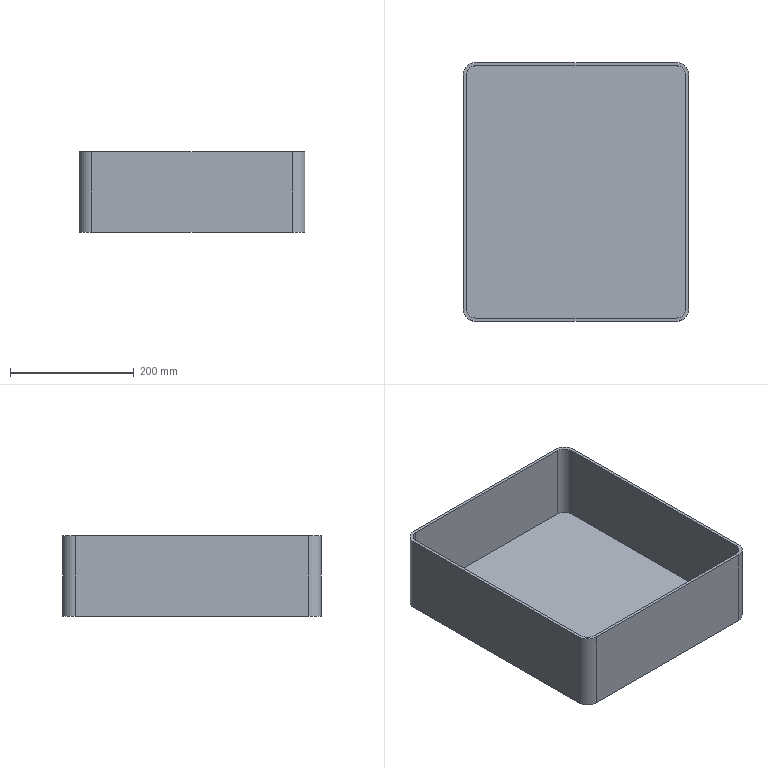Part | NX | features solid 2 | 1 solid | 19 faces | box 364.214 x 417 x 130 mm | volume 1702910 mm3 | plane 11 | cylinder 8 | commonest cylinder face diameters 30 x4 40 x4
STEP:
#1=CARTESIAN_POINT('',(-163.582,-691.316,-27.));
#2=VERTEX_POINT('',#1);
#3=CARTESIAN_POINT('',(160.632,-691.316,-27.));
#4=VERTEX_POINT('',#3);
#5=CARTESIAN_POINT('',(-1.475,-691.316,-27.));
#6=DIRECTION('',(-1.,0.,0.));
#7=VECTOR('',#6,1000.);
#8=LINE('',#5,#7);
#9=EDGE_CURVE('',#2,#4,#8,.F.);
#10=ORIENTED_EDGE('',*,*,#9,.F.);
#11=CARTESIAN_POINT('',(-183.582,-711.316,-27.));
#12=VERTEX_POINT('',#11);
#13=CARTESIAN_POINT('',(-163.582,-711.316,-27.));
#14=DIRECTION('',(0.,0.,-1.));
#15=DIRECTION('',(-1.,0.,0.));
#16=AXIS2_PLACEMENT_3D('',#13,#14,#15);
#17=CIRCLE('',#16,20.);
#18=EDGE_CURVE('',#2,#12,#17,.F.);
#19=ORIENTED_EDGE('',*,*,#18,.T.);
#20=CARTESIAN_POINT('',(-183.582,-1088.316,-27.));
#21=VERTEX_POINT('',#20);
#22=CARTESIAN_POINT('',(-183.582,-899.816,-27.));
#23=DIRECTION('',(0.,-1.,0.));
#24=VECTOR('',#23,1000.);
#25=LINE('',#22,#24);
#26=EDGE_CURVE('',#21,#12,#25,.F.);
#27=ORIENTED_EDGE('',*,*,#26,.F.);
#28=CARTESIAN_POINT('',(-163.582,-1108.316,-27.));
#29=VERTEX_POINT('',#28);
#30=CARTESIAN_POINT('',(-163.582,-1088.316,-27.));
#31=DIRECTION('',(0.,0.,-1.));
#32=DIRECTION('',(-1.,0.,0.));
#33=AXIS2_PLACEMENT_3D('',#30,#31,#32);
#34=CIRCLE('',#33,20.);
#35=EDGE_CURVE('',#21,#29,#34,.F.);
#36=ORIENTED_EDGE('',*,*,#35,.T.);
#37=CARTESIAN_POINT('',(160.632,-1108.316,-27.));
#38=VERTEX_POINT('',#37);
#39=CARTESIAN_POINT('',(-1.475,-1108.316,-27.));
#40=DIRECTION('',(1.,0.,0.));
#41=VECTOR('',#40,1000.);
#42=LINE('',#39,#41);
#43=EDGE_CURVE('',#38,#29,#42,.F.);
#44=ORIENTED_EDGE('',*,*,#43,.F.);
#45=CARTESIAN_POINT('',(180.632,-1088.316,-27.));
#46=VERTEX_POINT('',#45);
#47=CARTESIAN_POINT('',(160.632,-1088.316,-27.));
#48=DIRECTION('',(0.,0.,-1.));
#49=DIRECTION('',(-1.,0.,0.));
#50=AXIS2_PLACEMENT_3D('',#47,#48,#49);
#51=CIRCLE('',#50,20.);
#52=EDGE_CURVE('',#38,#46,#51,.F.);
#53=ORIENTED_EDGE('',*,*,#52,.T.);
#54=CARTESIAN_POINT('',(180.632,-711.316,-27.));
#55=VERTEX_POINT('',#54);
#56=CARTESIAN_POINT('',(180.632,-899.816,-27.));
#57=DIRECTION('',(0.,1.,0.));
#58=VECTOR('',#57,1000.);
#59=LINE('',#56,#58);
#60=EDGE_CURVE('',#55,#46,#59,.F.);
#61=ORIENTED_EDGE('',*,*,#60,.F.);
#62=CARTESIAN_POINT('',(160.632,-711.316,-27.));
#63=DIRECTION('',(0.,0.,-1.));
#64=DIRECTION('',(-1.,0.,0.));
#65=AXIS2_PLACEMENT_3D('',#62,#63,#64);
#66=CIRCLE('',#65,20.);
#67=EDGE_CURVE('',#55,#4,#66,.F.);
#68=ORIENTED_EDGE('',*,*,#67,.T.);
#69=EDGE_LOOP('',(#10,#19,#27,#36,#44,#53,#61,#68));
#70=FACE_BOUND('',#69,.T.);
#71=CARTESIAN_POINT('',(-163.582,-696.316,-27.));
#72=VERTEX_POINT('',#71);
#73=CARTESIAN_POINT('',(-178.582,-711.316,-27.));
#74=VERTEX_POINT('',#73);
#75=CARTESIAN_POINT('',(-163.582,-711.316,-27.));
#76=DIRECTION('',(0.,0.,-1.));
#77=DIRECTION('',(-1.,0.,0.));
#78=AXIS2_PLACEMENT_3D('',#75,#76,#77);
#79=CIRCLE('',#78,15.);
#80=EDGE_CURVE('',#72,#74,#79,.F.);
#81=ORIENTED_EDGE('',*,*,#80,.F.);
#82=CARTESIAN_POINT('',(160.632,-696.316,-27.));
#83=VERTEX_POINT('',#82);
#84=CARTESIAN_POINT('',(-1.475,-696.316,-27.));
#85=DIRECTION('',(-1.,0.,0.));
#86=VECTOR('',#85,1000.);
#87=LINE('',#84,#86);
#88=EDGE_CURVE('',#72,#83,#87,.F.);
#89=ORIENTED_EDGE('',*,*,#88,.T.);
#90=CARTESIAN_POINT('',(175.632,-711.316,-27.));
#91=VERTEX_POINT('',#90);
#92=CARTESIAN_POINT('',(160.632,-711.316,-27.));
#93=DIRECTION('',(0.,0.,-1.));
#94=DIRECTION('',(-1.,0.,0.));
#95=AXIS2_PLACEMENT_3D('',#92,#93,#94);
#96=CIRCLE('',#95,15.);
#97=EDGE_CURVE('',#91,#83,#96,.F.);
#98=ORIENTED_EDGE('',*,*,#97,.F.);
#99=CARTESIAN_POINT('',(175.632,-1088.316,-27.));
#100=VERTEX_POINT('',#99);
#101=CARTESIAN_POINT('',(175.632,-899.816,-27.));
#102=DIRECTION('',(0.,1.,0.));
#103=VECTOR('',#102,1000.);
#104=LINE('',#101,#103);
#105=EDGE_CURVE('',#91,#100,#104,.F.);
#106=ORIENTED_EDGE('',*,*,#105,.T.);
#107=CARTESIAN_POINT('',(160.632,-1103.316,-27.));
#108=VERTEX_POINT('',#107);
#109=CARTESIAN_POINT('',(160.632,-1088.316,-27.));
#110=DIRECTION('',(0.,0.,-1.));
#111=DIRECTION('',(-1.,0.,0.));
#112=AXIS2_PLACEMENT_3D('',#109,#110,#111);
#113=CIRCLE('',#112,15.);
#114=EDGE_CURVE('',#108,#100,#113,.F.);
#115=ORIENTED_EDGE('',*,*,#114,.F.);
#116=CARTESIAN_POINT('',(-163.582,-1103.316,-27.));
#117=VERTEX_POINT('',#116);
#118=CARTESIAN_POINT('',(-1.475,-1103.316,-27.));
#119=DIRECTION('',(1.,0.,0.));
#120=VECTOR('',#119,1000.);
#121=LINE('',#118,#120);
#122=EDGE_CURVE('',#108,#117,#121,.F.);
#123=ORIENTED_EDGE('',*,*,#122,.T.);
#124=CARTESIAN_POINT('',(-178.582,-1088.316,-27.));
#125=VERTEX_POINT('',#124);
#126=CARTESIAN_POINT('',(-163.582,-1088.316,-27.));
#127=DIRECTION('',(0.,0.,-1.));
#128=DIRECTION('',(-1.,0.,0.));
#129=AXIS2_PLACEMENT_3D('',#126,#127,#128);
#130=CIRCLE('',#129,15.);
#131=EDGE_CURVE('',#125,#117,#130,.F.);
#132=ORIENTED_EDGE('',*,*,#131,.F.);
#133=CARTESIAN_POINT('',(-178.582,-899.816,-27.));
#134=DIRECTION('',(0.,-1.,0.));
#135=VECTOR('',#134,1000.);
#136=LINE('',#133,#135);
#137=EDGE_CURVE('',#125,#74,#136,.F.);
#138=ORIENTED_EDGE('',*,*,#137,.T.);
#139=EDGE_LOOP('',(#81,#89,#98,#106,#115,#123,#132,#138));
#140=FACE_BOUND('',#139,.T.);
#141=CARTESIAN_POINT('',(193.825,-479.612,-27.));
#142=DIRECTION('',(0.,0.,-1.));
#143=DIRECTION('',(0.,1.,0.));
#144=AXIS2_PLACEMENT_3D('',#141,#142,#143);
#145=PLANE('',#144);
#146=ADVANCED_FACE('',(#70,#140),#145,.F.);
#147=CARTESIAN_POINT('',(-163.582,-1108.316,-157.));
#148=VERTEX_POINT('',#147);
#149=CARTESIAN_POINT('',(160.632,-1108.316,-157.));
#150=VERTEX_POINT('',#149);
#151=CARTESIAN_POINT('',(-1.475,-1108.316,-157.));
#152=DIRECTION('',(-1.,0.,0.));
#153=VECTOR('',#152,1000.);
#154=LINE('',#151,#153);
#155=EDGE_CURVE('',#148,#150,#154,.F.);
#156=ORIENTED_EDGE('',*,*,#155,.T.);
#157=CARTESIAN_POINT('',(160.632,-1108.316,-187.));
#158=DIRECTION('',(0.,0.,1.));
#159=VECTOR('',#158,1000.);
#160=LINE('',#157,#159);
#161=EDGE_CURVE('',#150,#38,#160,.T.);
#162=ORIENTED_EDGE('',*,*,#161,.T.);
#163=ORIENTED_EDGE('',*,*,#43,.T.);
#164=CARTESIAN_POINT('',(-163.582,-1108.316,-187.));
#165=DIRECTION('',(0.,0.,1.));
#166=VECTOR('',#165,1000.);
#167=LINE('',#164,#166);
#168=EDGE_CURVE('',#29,#148,#167,.F.);
#169=ORIENTED_EDGE('',*,*,#168,.T.);
#170=EDGE_LOOP('',(#156,#162,#163,#169));
#171=FACE_BOUND('',#170,.T.);
#172=CARTESIAN_POINT('',(-1.475,-1108.316,-187.));
#173=DIRECTION('',(0.,-1.,0.));
#174=DIRECTION('',(0.,0.,-1.));
#175=AXIS2_PLACEMENT_3D('',#172,#173,#174);
#176=PLANE('',#175);
#177=ADVANCED_FACE('',(#171),#176,.T.);
#178=ORIENTED_EDGE('',*,*,#26,.T.);
#179=CARTESIAN_POINT('',(-183.582,-711.316,-157.));
#180=VERTEX_POINT('',#179);
#181=CARTESIAN_POINT('',(-183.582,-711.316,-187.));
#182=DIRECTION('',(0.,0.,1.));
#183=VECTOR('',#182,1000.);
#184=LINE('',#181,#183);
#185=EDGE_CURVE('',#12,#180,#184,.F.);
#186=ORIENTED_EDGE('',*,*,#185,.T.);
#187=CARTESIAN_POINT('',(-183.582,-1088.316,-157.));
#188=VERTEX_POINT('',#187);
#189=CARTESIAN_POINT('',(-183.582,-899.816,-157.));
#190=DIRECTION('',(0.,1.,0.));
#191=VECTOR('',#190,1000.);
#192=LINE('',#189,#191);
#193=EDGE_CURVE('',#180,#188,#192,.F.);
#194=ORIENTED_EDGE('',*,*,#193,.T.);
#195=CARTESIAN_POINT('',(-183.582,-1088.316,-187.));
#196=DIRECTION('',(0.,0.,1.));
#197=VECTOR('',#196,1000.);
#198=LINE('',#195,#197);
#199=EDGE_CURVE('',#188,#21,#198,.T.);
#200=ORIENTED_EDGE('',*,*,#199,.T.);
#201=EDGE_LOOP('',(#178,#186,#194,#200));
#202=FACE_BOUND('',#201,.T.);
#203=CARTESIAN_POINT('',(-183.582,-899.816,-187.));
#204=DIRECTION('',(-1.,0.,0.));
#205=DIRECTION('',(0.,0.,1.));
#206=AXIS2_PLACEMENT_3D('',#203,#204,#205);
#207=PLANE('',#206);
#208=ADVANCED_FACE('',(#202),#207,.T.);
#209=CARTESIAN_POINT('',(160.632,-691.316,-157.));
#210=VERTEX_POINT('',#209);
#211=CARTESIAN_POINT('',(-163.582,-691.316,-157.));
#212=VERTEX_POINT('',#211);
#213=CARTESIAN_POINT('',(-1.475,-691.316,-157.));
#214=DIRECTION('',(1.,0.,0.));
#215=VECTOR('',#214,1000.);
#216=LINE('',#213,#215);
#217=EDGE_CURVE('',#210,#212,#216,.F.);
#218=ORIENTED_EDGE('',*,*,#217,.T.);
#219=CARTESIAN_POINT('',(-163.582,-691.316,-187.));
#220=DIRECTION('',(0.,0.,1.));
#221=VECTOR('',#220,1000.);
#222=LINE('',#219,#221);
#223=EDGE_CURVE('',#212,#2,#222,.T.);
#224=ORIENTED_EDGE('',*,*,#223,.T.);
#225=ORIENTED_EDGE('',*,*,#9,.T.);
#226=CARTESIAN_POINT('',(160.632,-691.316,-187.));
#227=DIRECTION('',(0.,0.,1.));
#228=VECTOR('',#227,1000.);
#229=LINE('',#226,#228);
#230=EDGE_CURVE('',#4,#210,#229,.F.);
#231=ORIENTED_EDGE('',*,*,#230,.T.);
#232=EDGE_LOOP('',(#218,#224,#225,#231));
#233=FACE_BOUND('',#232,.T.);
#234=CARTESIAN_POINT('',(-1.475,-691.316,-187.));
#235=DIRECTION('',(0.,1.,0.));
#236=DIRECTION('',(0.,0.,1.));
#237=AXIS2_PLACEMENT_3D('',#234,#235,#236);
#238=PLANE('',#237);
#239=ADVANCED_FACE('',(#233),#238,.T.);
#240=ORIENTED_EDGE('',*,*,#193,.F.);
#241=CARTESIAN_POINT('',(-163.582,-711.316,-157.));
#242=DIRECTION('',(0.,0.,1.));
#243=DIRECTION('',(1.,0.,0.));
#244=AXIS2_PLACEMENT_3D('',#241,#242,#243);
#245=CIRCLE('',#244,20.);
#246=EDGE_CURVE('',#180,#212,#245,.F.);
#247=ORIENTED_EDGE('',*,*,#246,.T.);
#248=ORIENTED_EDGE('',*,*,#217,.F.);
#249=CARTESIAN_POINT('',(180.632,-711.316,-157.));
#250=VERTEX_POINT('',#249);
#251=CARTESIAN_POINT('',(160.632,-711.316,-157.));
#252=DIRECTION('',(0.,0.,1.));
#253=DIRECTION('',(1.,0.,0.));
#254=AXIS2_PLACEMENT_3D('',#251,#252,#253);
#255=CIRCLE('',#254,20.);
#256=EDGE_CURVE('',#210,#250,#255,.F.);
#257=ORIENTED_EDGE('',*,*,#256,.T.);
#258=CARTESIAN_POINT('',(180.632,-1088.316,-157.));
#259=VERTEX_POINT('',#258);
#260=CARTESIAN_POINT('',(180.632,-899.816,-157.));
#261=DIRECTION('',(0.,-1.,0.));
#262=VECTOR('',#261,1000.);
#263=LINE('',#260,#262);
#264=EDGE_CURVE('',#259,#250,#263,.F.);
#265=ORIENTED_EDGE('',*,*,#264,.F.);
#266=CARTESIAN_POINT('',(160.632,-1088.316,-157.));
#267=DIRECTION('',(0.,0.,1.));
#268=DIRECTION('',(1.,0.,0.));
#269=AXIS2_PLACEMENT_3D('',#266,#267,#268);
#270=CIRCLE('',#269,20.);
#271=EDGE_CURVE('',#259,#150,#270,.F.);
#272=ORIENTED_EDGE('',*,*,#271,.T.);
#273=ORIENTED_EDGE('',*,*,#155,.F.);
#274=CARTESIAN_POINT('',(-163.582,-1088.316,-157.));
#275=DIRECTION('',(0.,0.,1.));
#276=DIRECTION('',(1.,0.,0.));
#277=AXIS2_PLACEMENT_3D('',#274,#275,#276);
#278=CIRCLE('',#277,20.);
#279=EDGE_CURVE('',#148,#188,#278,.F.);
#280=ORIENTED_EDGE('',*,*,#279,.T.);
#281=EDGE_LOOP('',(#240,#247,#248,#257,#265,#272,#273,#280));
#282=FACE_BOUND('',#281,.T.);
#283=CARTESIAN_POINT('',(174.525,-16.,-157.));
#284=DIRECTION('',(0.,0.,1.));
#285=DIRECTION('',(-1.,0.,0.));
#286=AXIS2_PLACEMENT_3D('',#283,#284,#285);
#287=PLANE('',#286);
#288=ADVANCED_FACE('',(#282),#287,.F.);
#289=ORIENTED_EDGE('',*,*,#264,.T.);
#290=CARTESIAN_POINT('',(180.632,-711.316,-187.));
#291=DIRECTION('',(0.,0.,1.));
#292=VECTOR('',#291,1000.);
#293=LINE('',#290,#292);
#294=EDGE_CURVE('',#250,#55,#293,.T.);
#295=ORIENTED_EDGE('',*,*,#294,.T.);
#296=ORIENTED_EDGE('',*,*,#60,.T.);
#297=CARTESIAN_POINT('',(180.632,-1088.316,-187.));
#298=DIRECTION('',(0.,0.,1.));
#299=VECTOR('',#298,1000.);
#300=LINE('',#297,#299);
#301=EDGE_CURVE('',#46,#259,#300,.F.);
#302=ORIENTED_EDGE('',*,*,#301,.T.);
#303=EDGE_LOOP('',(#289,#295,#296,#302));
#304=FACE_BOUND('',#303,.T.);
#305=CARTESIAN_POINT('',(180.632,-899.816,-187.));
#306=DIRECTION('',(1.,0.,0.));
#307=DIRECTION('',(0.,0.,-1.));
#308=AXIS2_PLACEMENT_3D('',#305,#306,#307);
#309=PLANE('',#308);
#310=ADVANCED_FACE('',(#304),#309,.T.);
#311=ORIENTED_EDGE('',*,*,#246,.F.);
#312=ORIENTED_EDGE('',*,*,#185,.F.);
#313=ORIENTED_EDGE('',*,*,#18,.F.);
#314=ORIENTED_EDGE('',*,*,#223,.F.);
#315=EDGE_LOOP('',(#311,#312,#313,#314));
#316=FACE_BOUND('',#315,.T.);
#317=CARTESIAN_POINT('',(-163.582,-711.316,-187.));
#318=DIRECTION('',(0.,0.,1.));
#319=DIRECTION('',(1.,0.,0.));
#320=AXIS2_PLACEMENT_3D('',#317,#318,#319);
#321=CYLINDRICAL_SURFACE('',#320,20.);
#322=ADVANCED_FACE('',(#316),#321,.T.);
#323=ORIENTED_EDGE('',*,*,#256,.F.);
#324=ORIENTED_EDGE('',*,*,#230,.F.);
#325=ORIENTED_EDGE('',*,*,#67,.F.);
#326=ORIENTED_EDGE('',*,*,#294,.F.);
#327=EDGE_LOOP('',(#323,#324,#325,#326));
#328=FACE_BOUND('',#327,.T.);
#329=CARTESIAN_POINT('',(160.632,-711.316,-187.));
#330=DIRECTION('',(0.,0.,1.));
#331=DIRECTION('',(1.,0.,0.));
#332=AXIS2_PLACEMENT_3D('',#329,#330,#331);
#333=CYLINDRICAL_SURFACE('',#332,20.);
#334=ADVANCED_FACE('',(#328),#333,.T.);
#335=ORIENTED_EDGE('',*,*,#271,.F.);
#336=ORIENTED_EDGE('',*,*,#301,.F.);
#337=ORIENTED_EDGE('',*,*,#52,.F.);
#338=ORIENTED_EDGE('',*,*,#161,.F.);
#339=EDGE_LOOP('',(#335,#336,#337,#338));
#340=FACE_BOUND('',#339,.T.);
#341=CARTESIAN_POINT('',(160.632,-1088.316,-187.));
#342=DIRECTION('',(0.,0.,1.));
#343=DIRECTION('',(1.,0.,0.));
#344=AXIS2_PLACEMENT_3D('',#341,#342,#343);
#345=CYLINDRICAL_SURFACE('',#344,20.);
#346=ADVANCED_FACE('',(#340),#345,.T.);
#347=ORIENTED_EDGE('',*,*,#279,.F.);
#348=ORIENTED_EDGE('',*,*,#168,.F.);
#349=ORIENTED_EDGE('',*,*,#35,.F.);
#350=ORIENTED_EDGE('',*,*,#199,.F.);
#351=EDGE_LOOP('',(#347,#348,#349,#350));
#352=FACE_BOUND('',#351,.T.);
#353=CARTESIAN_POINT('',(-163.582,-1088.316,-187.));
#354=DIRECTION('',(0.,0.,1.));
#355=DIRECTION('',(1.,0.,0.));
#356=AXIS2_PLACEMENT_3D('',#353,#354,#355);
#357=CYLINDRICAL_SURFACE('',#356,20.);
#358=ADVANCED_FACE('',(#352),#357,.T.);
#359=CARTESIAN_POINT('',(-163.582,-1103.316,-152.));
#360=VERTEX_POINT('',#359);
#361=CARTESIAN_POINT('',(160.632,-1103.316,-152.));
#362=VERTEX_POINT('',#361);
#363=CARTESIAN_POINT('',(-1.475,-1103.316,-152.));
#364=DIRECTION('',(-1.,0.,0.));
#365=VECTOR('',#364,1000.);
#366=LINE('',#363,#365);
#367=EDGE_CURVE('',#360,#362,#366,.F.);
#368=ORIENTED_EDGE('',*,*,#367,.F.);
#369=CARTESIAN_POINT('',(-163.582,-1103.316,-187.));
#370=DIRECTION('',(0.,0.,-1.));
#371=VECTOR('',#370,1000.);
#372=LINE('',#369,#371);
#373=EDGE_CURVE('',#117,#360,#372,.T.);
#374=ORIENTED_EDGE('',*,*,#373,.F.);
#375=ORIENTED_EDGE('',*,*,#122,.F.);
#376=CARTESIAN_POINT('',(160.632,-1103.316,-187.));
#377=DIRECTION('',(0.,0.,-1.));
#378=VECTOR('',#377,1000.);
#379=LINE('',#376,#378);
#380=EDGE_CURVE('',#362,#108,#379,.F.);
#381=ORIENTED_EDGE('',*,*,#380,.F.);
#382=EDGE_LOOP('',(#368,#374,#375,#381));
#383=FACE_BOUND('',#382,.T.);
#384=CARTESIAN_POINT('',(-1.475,-1103.316,-187.));
#385=DIRECTION('',(0.,-1.,0.));
#386=DIRECTION('',(0.,0.,-1.));
#387=AXIS2_PLACEMENT_3D('',#384,#385,#386);
#388=PLANE('',#387);
#389=ADVANCED_FACE('',(#383),#388,.F.);
#390=ORIENTED_EDGE('',*,*,#137,.F.);
#391=CARTESIAN_POINT('',(-178.582,-1088.316,-152.));
#392=VERTEX_POINT('',#391);
#393=CARTESIAN_POINT('',(-178.582,-1088.316,-187.));
#394=DIRECTION('',(0.,0.,1.));
#395=VECTOR('',#394,1000.);
#396=LINE('',#393,#395);
#397=EDGE_CURVE('',#392,#125,#396,.T.);
#398=ORIENTED_EDGE('',*,*,#397,.F.);
#399=CARTESIAN_POINT('',(-178.582,-711.316,-152.));
#400=VERTEX_POINT('',#399);
#401=CARTESIAN_POINT('',(-178.582,-899.816,-152.));
#402=DIRECTION('',(0.,1.,0.));
#403=VECTOR('',#402,1000.);
#404=LINE('',#401,#403);
#405=EDGE_CURVE('',#400,#392,#404,.F.);
#406=ORIENTED_EDGE('',*,*,#405,.F.);
#407=CARTESIAN_POINT('',(-178.582,-711.316,-187.));
#408=DIRECTION('',(0.,0.,1.));
#409=VECTOR('',#408,1000.);
#410=LINE('',#407,#409);
#411=EDGE_CURVE('',#74,#400,#410,.F.);
#412=ORIENTED_EDGE('',*,*,#411,.F.);
#413=EDGE_LOOP('',(#390,#398,#406,#412));
#414=FACE_BOUND('',#413,.T.);
#415=CARTESIAN_POINT('',(-178.582,-899.816,-187.));
#416=DIRECTION('',(-1.,0.,0.));
#417=DIRECTION('',(0.,0.,1.));
#418=AXIS2_PLACEMENT_3D('',#415,#416,#417);
#419=PLANE('',#418);
#420=ADVANCED_FACE('',(#414),#419,.F.);
#421=CARTESIAN_POINT('',(160.632,-696.316,-152.));
#422=VERTEX_POINT('',#421);
#423=CARTESIAN_POINT('',(-163.582,-696.316,-152.));
#424=VERTEX_POINT('',#423);
#425=CARTESIAN_POINT('',(-1.475,-696.316,-152.));
#426=DIRECTION('',(1.,0.,0.));
#427=VECTOR('',#426,1000.);
#428=LINE('',#425,#427);
#429=EDGE_CURVE('',#422,#424,#428,.F.);
#430=ORIENTED_EDGE('',*,*,#429,.F.);
#431=CARTESIAN_POINT('',(160.632,-696.316,-187.));
#432=DIRECTION('',(0.,0.,1.));
#433=VECTOR('',#432,1000.);
#434=LINE('',#431,#433);
#435=EDGE_CURVE('',#83,#422,#434,.F.);
#436=ORIENTED_EDGE('',*,*,#435,.F.);
#437=ORIENTED_EDGE('',*,*,#88,.F.);
#438=CARTESIAN_POINT('',(-163.582,-696.316,-187.));
#439=DIRECTION('',(0.,0.,1.));
#440=VECTOR('',#439,1000.);
#441=LINE('',#438,#440);
#442=EDGE_CURVE('',#424,#72,#441,.T.);
#443=ORIENTED_EDGE('',*,*,#442,.F.);
#444=EDGE_LOOP('',(#430,#436,#437,#443));
#445=FACE_BOUND('',#444,.T.);
#446=CARTESIAN_POINT('',(-1.475,-696.316,-187.));
#447=DIRECTION('',(0.,1.,0.));
#448=DIRECTION('',(0.,0.,1.));
#449=AXIS2_PLACEMENT_3D('',#446,#447,#448);
#450=PLANE('',#449);
#451=ADVANCED_FACE('',(#445),#450,.F.);
#452=ORIENTED_EDGE('',*,*,#405,.T.);
#453=CARTESIAN_POINT('',(-163.582,-1088.316,-152.));
#454=DIRECTION('',(0.,0.,1.));
#455=DIRECTION('',(1.,0.,0.));
#456=AXIS2_PLACEMENT_3D('',#453,#454,#455);
#457=CIRCLE('',#456,15.);
#458=EDGE_CURVE('',#360,#392,#457,.F.);
#459=ORIENTED_EDGE('',*,*,#458,.F.);
#460=ORIENTED_EDGE('',*,*,#367,.T.);
#461=CARTESIAN_POINT('',(175.632,-1088.316,-152.));
#462=VERTEX_POINT('',#461);
#463=CARTESIAN_POINT('',(160.632,-1088.316,-152.));
#464=DIRECTION('',(0.,0.,1.));
#465=DIRECTION('',(1.,0.,0.));
#466=AXIS2_PLACEMENT_3D('',#463,#464,#465);
#467=CIRCLE('',#466,15.);
#468=EDGE_CURVE('',#462,#362,#467,.F.);
#469=ORIENTED_EDGE('',*,*,#468,.F.);
#470=CARTESIAN_POINT('',(175.632,-711.316,-152.));
#471=VERTEX_POINT('',#470);
#472=CARTESIAN_POINT('',(175.632,-899.816,-152.));
#473=DIRECTION('',(0.,-1.,0.));
#474=VECTOR('',#473,1000.);
#475=LINE('',#472,#474);
#476=EDGE_CURVE('',#462,#471,#475,.F.);
#477=ORIENTED_EDGE('',*,*,#476,.T.);
#478=CARTESIAN_POINT('',(160.632,-711.316,-152.));
#479=DIRECTION('',(0.,0.,1.));
#480=DIRECTION('',(1.,0.,0.));
#481=AXIS2_PLACEMENT_3D('',#478,#479,#480);
#482=CIRCLE('',#481,15.);
#483=EDGE_CURVE('',#422,#471,#482,.F.);
#484=ORIENTED_EDGE('',*,*,#483,.F.);
#485=ORIENTED_EDGE('',*,*,#429,.T.);
#486=CARTESIAN_POINT('',(-163.582,-711.316,-152.));
#487=DIRECTION('',(0.,0.,1.));
#488=DIRECTION('',(1.,0.,0.));
#489=AXIS2_PLACEMENT_3D('',#486,#487,#488);
#490=CIRCLE('',#489,15.);
#491=EDGE_CURVE('',#400,#424,#490,.F.);
#492=ORIENTED_EDGE('',*,*,#491,.F.);
#493=EDGE_LOOP('',(#452,#459,#460,#469,#477,#484,#485,#492));
#494=FACE_BOUND('',#493,.T.);
#495=CARTESIAN_POINT('',(174.525,-16.,-152.));
#496=DIRECTION('',(0.,0.,1.));
#497=DIRECTION('',(-1.,0.,0.));
#498=AXIS2_PLACEMENT_3D('',#495,#496,#497);
#499=PLANE('',#498);
#500=ADVANCED_FACE('',(#494),#499,.T.);
#501=ORIENTED_EDGE('',*,*,#476,.F.);
#502=CARTESIAN_POINT('',(175.632,-1088.316,-187.));
#503=DIRECTION('',(0.,0.,-1.));
#504=VECTOR('',#503,1000.);
#505=LINE('',#502,#504);
#506=EDGE_CURVE('',#100,#462,#505,.T.);
#507=ORIENTED_EDGE('',*,*,#506,.F.);
#508=ORIENTED_EDGE('',*,*,#105,.F.);
#509=CARTESIAN_POINT('',(175.632,-711.316,-187.));
#510=DIRECTION('',(0.,0.,-1.));
#511=VECTOR('',#510,1000.);
#512=LINE('',#509,#511);
#513=EDGE_CURVE('',#471,#91,#512,.F.);
#514=ORIENTED_EDGE('',*,*,#513,.F.);
#515=EDGE_LOOP('',(#501,#507,#508,#514));
#516=FACE_BOUND('',#515,.T.);
#517=CARTESIAN_POINT('',(175.632,-899.816,-187.));
#518=DIRECTION('',(1.,0.,0.));
#519=DIRECTION('',(0.,0.,-1.));
#520=AXIS2_PLACEMENT_3D('',#517,#518,#519);
#521=PLANE('',#520);
#522=ADVANCED_FACE('',(#516),#521,.F.);
#523=ORIENTED_EDGE('',*,*,#491,.T.);
#524=ORIENTED_EDGE('',*,*,#442,.T.);
#525=ORIENTED_EDGE('',*,*,#80,.T.);
#526=ORIENTED_EDGE('',*,*,#411,.T.);
#527=EDGE_LOOP('',(#523,#524,#525,#526));
#528=FACE_BOUND('',#527,.T.);
#529=CARTESIAN_POINT('',(-163.582,-711.316,-187.));
#530=DIRECTION('',(0.,0.,1.));
#531=DIRECTION('',(1.,0.,0.));
#532=AXIS2_PLACEMENT_3D('',#529,#530,#531);
#533=CYLINDRICAL_SURFACE('',#532,15.);
#534=ADVANCED_FACE('',(#528),#533,.F.);
#535=ORIENTED_EDGE('',*,*,#483,.T.);
#536=ORIENTED_EDGE('',*,*,#513,.T.);
#537=ORIENTED_EDGE('',*,*,#97,.T.);
#538=ORIENTED_EDGE('',*,*,#435,.T.);
#539=EDGE_LOOP('',(#535,#536,#537,#538));
#540=FACE_BOUND('',#539,.T.);
#541=CARTESIAN_POINT('',(160.632,-711.316,-187.));
#542=DIRECTION('',(0.,0.,1.));
#543=DIRECTION('',(1.,0.,0.));
#544=AXIS2_PLACEMENT_3D('',#541,#542,#543);
#545=CYLINDRICAL_SURFACE('',#544,15.);
#546=ADVANCED_FACE('',(#540),#545,.F.);
#547=ORIENTED_EDGE('',*,*,#468,.T.);
#548=ORIENTED_EDGE('',*,*,#380,.T.);
#549=ORIENTED_EDGE('',*,*,#114,.T.);
#550=ORIENTED_EDGE('',*,*,#506,.T.);
#551=EDGE_LOOP('',(#547,#548,#549,#550));
#552=FACE_BOUND('',#551,.T.);
#553=CARTESIAN_POINT('',(160.632,-1088.316,-187.));
#554=DIRECTION('',(0.,0.,1.));
#555=DIRECTION('',(1.,0.,0.));
#556=AXIS2_PLACEMENT_3D('',#553,#554,#555);
#557=CYLINDRICAL_SURFACE('',#556,15.);
#558=ADVANCED_FACE('',(#552),#557,.F.);
#559=ORIENTED_EDGE('',*,*,#458,.T.);
#560=ORIENTED_EDGE('',*,*,#397,.T.);
#561=ORIENTED_EDGE('',*,*,#131,.T.);
#562=ORIENTED_EDGE('',*,*,#373,.T.);
#563=EDGE_LOOP('',(#559,#560,#561,#562));
#564=FACE_BOUND('',#563,.T.);
#565=CARTESIAN_POINT('',(-163.582,-1088.316,-187.));
#566=DIRECTION('',(0.,0.,1.));
#567=DIRECTION('',(1.,0.,0.));
#568=AXIS2_PLACEMENT_3D('',#565,#566,#567);
#569=CYLINDRICAL_SURFACE('',#568,15.);
#570=ADVANCED_FACE('',(#564),#569,.F.);
#571=CLOSED_SHELL('',(#146,#177,#208,#239,#288,#310,#322,#334,#346,#358,#389,#420,#451,#500,#522,#534,#546,#558,#570));
#572=MANIFOLD_SOLID_BREP('',#571);
#573=(LENGTH_UNIT()NAMED_UNIT(*)SI_UNIT(.MILLI.,.METRE.));
#574=UNCERTAINTY_MEASURE_WITH_UNIT(LENGTH_MEASURE(0.00001),#573,'','');
#575=(NAMED_UNIT(*)PLANE_ANGLE_UNIT()SI_UNIT($,.RADIAN.));
#576=(NAMED_UNIT(*)SI_UNIT($,.STERADIAN.)SOLID_ANGLE_UNIT());
#577=(GEOMETRIC_REPRESENTATION_CONTEXT(3)GLOBAL_UNCERTAINTY_ASSIGNED_CONTEXT((#574))GLOBAL_UNIT_ASSIGNED_CONTEXT((#573,#575,#576))REPRESENTATION_CONTEXT('',''));
#578=ADVANCED_BREP_SHAPE_REPRESENTATION('',(#572),#577);